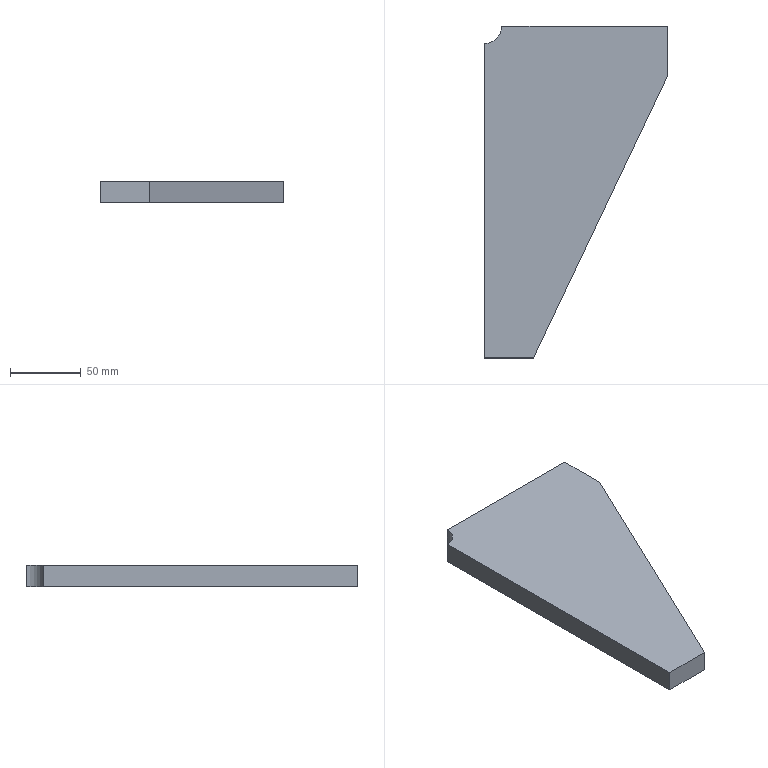Part | STEP file | Input 76 | 1 solid | 8 faces | box 130 x 235 x 15 mm | volume 313909 mm3 | plane 7 | cylinder 1 | commonest cylinder face diameters 25 x1
STEP:
#1=CARTESIAN_POINT('',(0.,0.,0.));
#2=DIRECTION('',(0.,0.,1.));
#3=DIRECTION('',(1.,0.,0.));
#4=AXIS2_PLACEMENT_3D('',#1,#2,#3);
#5=CARTESIAN_POINT('',(4022.,160.,7.5));
#6=VERTEX_POINT('',#5);
#7=CARTESIAN_POINT('',(4057.,160.,7.5));
#8=VERTEX_POINT('',#7);
#9=CARTESIAN_POINT('',(4057.,160.,7.5));
#10=DIRECTION('',(1.,0.,0.));
#11=VECTOR('',#10,1.);
#12=LINE('',#9,#11);
#13=CARTESIAN_POINT('',(4057.,160.,-7.5));
#14=DIRECTION('',(0.,-1.,0.));
#15=DIRECTION('',(1.,0.,0.));
#16=AXIS2_PLACEMENT_3D('',#13,#14,#15);
#17=PLANE('',#16);
#18=CARTESIAN_POINT('',(0.,15.));
#19=DIRECTION('',(1.,0.));
#20=VECTOR('',#19,1.);
#21=LINE('',#18,#20);
#22=(GEOMETRIC_REPRESENTATION_CONTEXT(2)PARAMETRIC_REPRESENTATION_CONTEXT()REPRESENTATION_CONTEXT('',''));
#23=DEFINITIONAL_REPRESENTATION('',(#21),#22);
#24=PCURVE('',#17,#23);
#25=CARTESIAN_POINT('',(4022.,395.,7.5));
#26=DIRECTION('',(0.,0.,1.));
#27=DIRECTION('',(1.,0.,0.));
#28=AXIS2_PLACEMENT_3D('',#25,#26,#27);
#29=PLANE('',#28);
#30=CARTESIAN_POINT('',(35.,-235.));
#31=DIRECTION('',(1.,0.));
#32=VECTOR('',#31,1.);
#33=LINE('',#30,#32);
#34=(GEOMETRIC_REPRESENTATION_CONTEXT(2)PARAMETRIC_REPRESENTATION_CONTEXT()REPRESENTATION_CONTEXT('',''));
#35=DEFINITIONAL_REPRESENTATION('',(#33),#34);
#36=PCURVE('',#29,#35);
#37=SURFACE_CURVE('',#12,(#24,#36),.PCURVE_S1.);
#38=EDGE_CURVE('',#6,#8,#37,.T.);
#39=ORIENTED_EDGE('',*,*,#38,.F.);
#40=CARTESIAN_POINT('',(4022.,160.,-7.5));
#41=VERTEX_POINT('',#40);
#42=CARTESIAN_POINT('',(4022.,160.,-7.5));
#43=DIRECTION('',(0.,0.,1.));
#44=VECTOR('',#43,1.);
#45=LINE('',#42,#44);
#46=CARTESIAN_POINT('',(-35.,0.));
#47=DIRECTION('',(0.,1.));
#48=VECTOR('',#47,1.);
#49=LINE('',#46,#48);
#50=(GEOMETRIC_REPRESENTATION_CONTEXT(2)PARAMETRIC_REPRESENTATION_CONTEXT()REPRESENTATION_CONTEXT('',''));
#51=DEFINITIONAL_REPRESENTATION('',(#49),#50);
#52=PCURVE('',#17,#51);
#53=CARTESIAN_POINT('',(4022.,160.,-7.5));
#54=DIRECTION('',(-1.,0.,0.));
#55=DIRECTION('',(0.,0.,1.));
#56=AXIS2_PLACEMENT_3D('',#53,#54,#55);
#57=PLANE('',#56);
#58=CARTESIAN_POINT('',(0.,0.));
#59=DIRECTION('',(1.,0.));
#60=VECTOR('',#59,1.);
#61=LINE('',#58,#60);
#62=(GEOMETRIC_REPRESENTATION_CONTEXT(2)PARAMETRIC_REPRESENTATION_CONTEXT()REPRESENTATION_CONTEXT('',''));
#63=DEFINITIONAL_REPRESENTATION('',(#61),#62);
#64=PCURVE('',#57,#63);
#65=SURFACE_CURVE('',#45,(#52,#64),.PCURVE_S1.);
#66=EDGE_CURVE('',#41,#6,#65,.T.);
#67=ORIENTED_EDGE('',*,*,#66,.F.);
#68=CARTESIAN_POINT('',(4057.,160.,-7.5));
#69=VERTEX_POINT('',#68);
#70=CARTESIAN_POINT('',(4057.,160.,-7.5));
#71=DIRECTION('',(1.,0.,0.));
#72=VECTOR('',#71,1.);
#73=LINE('',#70,#72);
#74=CARTESIAN_POINT('',(0.,0.));
#75=DIRECTION('',(1.,0.));
#76=VECTOR('',#75,1.);
#77=LINE('',#74,#76);
#78=(GEOMETRIC_REPRESENTATION_CONTEXT(2)PARAMETRIC_REPRESENTATION_CONTEXT()REPRESENTATION_CONTEXT('',''));
#79=DEFINITIONAL_REPRESENTATION('',(#77),#78);
#80=PCURVE('',#17,#79);
#81=CARTESIAN_POINT('',(4022.,395.,-7.5));
#82=DIRECTION('',(0.,0.,1.));
#83=DIRECTION('',(1.,0.,0.));
#84=AXIS2_PLACEMENT_3D('',#81,#82,#83);
#85=PLANE('',#84);
#86=CARTESIAN_POINT('',(35.,-235.));
#87=DIRECTION('',(1.,0.));
#88=VECTOR('',#87,1.);
#89=LINE('',#86,#88);
#90=(GEOMETRIC_REPRESENTATION_CONTEXT(2)PARAMETRIC_REPRESENTATION_CONTEXT()REPRESENTATION_CONTEXT('',''));
#91=DEFINITIONAL_REPRESENTATION('',(#89),#90);
#92=PCURVE('',#85,#91);
#93=SURFACE_CURVE('',#73,(#80,#92),.PCURVE_S1.);
#94=EDGE_CURVE('',#41,#69,#93,.T.);
#95=ORIENTED_EDGE('',*,*,#94,.T.);
#96=CARTESIAN_POINT('',(4057.,160.,-7.5));
#97=DIRECTION('',(0.,0.,1.));
#98=VECTOR('',#97,1.);
#99=LINE('',#96,#98);
#100=CARTESIAN_POINT('',(0.,0.));
#101=DIRECTION('',(0.,1.));
#102=VECTOR('',#101,1.);
#103=LINE('',#100,#102);
#104=(GEOMETRIC_REPRESENTATION_CONTEXT(2)PARAMETRIC_REPRESENTATION_CONTEXT()REPRESENTATION_CONTEXT('',''));
#105=DEFINITIONAL_REPRESENTATION('',(#103),#104);
#106=PCURVE('',#17,#105);
#107=CARTESIAN_POINT('',(4152.,360.,-7.5));
#108=DIRECTION('',(0.9033,-0.4291,0.));
#109=DIRECTION('',(0.4291,0.9033,0.));
#110=AXIS2_PLACEMENT_3D('',#107,#108,#109);
#111=PLANE('',#110);
#112=CARTESIAN_POINT('',(-221.416,0.));
#113=DIRECTION('',(0.,1.));
#114=VECTOR('',#113,1.);
#115=LINE('',#112,#114);
#116=(GEOMETRIC_REPRESENTATION_CONTEXT(2)PARAMETRIC_REPRESENTATION_CONTEXT()REPRESENTATION_CONTEXT('',''));
#117=DEFINITIONAL_REPRESENTATION('',(#115),#116);
#118=PCURVE('',#111,#117);
#119=SURFACE_CURVE('',#99,(#106,#118),.PCURVE_S1.);
#120=EDGE_CURVE('',#69,#8,#119,.T.);
#121=ORIENTED_EDGE('',*,*,#120,.T.);
#122=EDGE_LOOP('',(#39,#67,#95,#121));
#123=FACE_BOUND('',#122,.T.);
#124=ADVANCED_FACE('',(#123),#17,.T.);
#125=CARTESIAN_POINT('',(4022.,382.5,7.5));
#126=VERTEX_POINT('',#125);
#127=CARTESIAN_POINT('',(4022.,160.,7.5));
#128=DIRECTION('',(0.,-1.,0.));
#129=VECTOR('',#128,1.);
#130=LINE('',#127,#129);
#131=CARTESIAN_POINT('',(15.,0.));
#132=DIRECTION('',(0.,-1.));
#133=VECTOR('',#132,1.);
#134=LINE('',#131,#133);
#135=(GEOMETRIC_REPRESENTATION_CONTEXT(2)PARAMETRIC_REPRESENTATION_CONTEXT()REPRESENTATION_CONTEXT('',''));
#136=DEFINITIONAL_REPRESENTATION('',(#134),#135);
#137=PCURVE('',#57,#136);
#138=CARTESIAN_POINT('',(0.,-235.));
#139=DIRECTION('',(0.,-1.));
#140=VECTOR('',#139,1.);
#141=LINE('',#138,#140);
#142=(GEOMETRIC_REPRESENTATION_CONTEXT(2)PARAMETRIC_REPRESENTATION_CONTEXT()REPRESENTATION_CONTEXT('',''));
#143=DEFINITIONAL_REPRESENTATION('',(#141),#142);
#144=PCURVE('',#29,#143);
#145=SURFACE_CURVE('',#130,(#137,#144),.PCURVE_S1.);
#146=EDGE_CURVE('',#126,#6,#145,.T.);
#147=ORIENTED_EDGE('',*,*,#146,.F.);
#148=CARTESIAN_POINT('',(4022.,382.5,-7.5));
#149=VERTEX_POINT('',#148);
#150=CARTESIAN_POINT('',(4022.,382.5,-7.5));
#151=DIRECTION('',(0.,0.,1.));
#152=VECTOR('',#151,1.);
#153=LINE('',#150,#152);
#154=CARTESIAN_POINT('',(0.,222.5));
#155=DIRECTION('',(1.,0.));
#156=VECTOR('',#155,1.);
#157=LINE('',#154,#156);
#158=(GEOMETRIC_REPRESENTATION_CONTEXT(2)PARAMETRIC_REPRESENTATION_CONTEXT()REPRESENTATION_CONTEXT('',''));
#159=DEFINITIONAL_REPRESENTATION('',(#157),#158);
#160=PCURVE('',#57,#159);
#161=CARTESIAN_POINT('',(4022.,395.,-7.5));
#162=DIRECTION('',(0.,0.,1.));
#163=DIRECTION('',(1.,0.,0.));
#164=AXIS2_PLACEMENT_3D('',#161,#162,#163);
#165=CYLINDRICAL_SURFACE('',#164,12.5);
#166=CARTESIAN_POINT('',(4.712,0.));
#167=DIRECTION('',(0.,1.));
#168=VECTOR('',#167,1.);
#169=LINE('',#166,#168);
#170=(GEOMETRIC_REPRESENTATION_CONTEXT(2)PARAMETRIC_REPRESENTATION_CONTEXT()REPRESENTATION_CONTEXT('',''));
#171=DEFINITIONAL_REPRESENTATION('',(#169),#170);
#172=PCURVE('',#165,#171);
#173=SURFACE_CURVE('',#153,(#160,#172),.PCURVE_S1.);
#174=EDGE_CURVE('',#149,#126,#173,.T.);
#175=ORIENTED_EDGE('',*,*,#174,.F.);
#176=CARTESIAN_POINT('',(4022.,160.,-7.5));
#177=DIRECTION('',(0.,-1.,0.));
#178=VECTOR('',#177,1.);
#179=LINE('',#176,#178);
#180=CARTESIAN_POINT('',(0.,0.));
#181=DIRECTION('',(0.,-1.));
#182=VECTOR('',#181,1.);
#183=LINE('',#180,#182);
#184=(GEOMETRIC_REPRESENTATION_CONTEXT(2)PARAMETRIC_REPRESENTATION_CONTEXT()REPRESENTATION_CONTEXT('',''));
#185=DEFINITIONAL_REPRESENTATION('',(#183),#184);
#186=PCURVE('',#57,#185);
#187=CARTESIAN_POINT('',(0.,-235.));
#188=DIRECTION('',(0.,-1.));
#189=VECTOR('',#188,1.);
#190=LINE('',#187,#189);
#191=(GEOMETRIC_REPRESENTATION_CONTEXT(2)PARAMETRIC_REPRESENTATION_CONTEXT()REPRESENTATION_CONTEXT('',''));
#192=DEFINITIONAL_REPRESENTATION('',(#190),#191);
#193=PCURVE('',#85,#192);
#194=SURFACE_CURVE('',#179,(#186,#193),.PCURVE_S1.);
#195=EDGE_CURVE('',#149,#41,#194,.T.);
#196=ORIENTED_EDGE('',*,*,#195,.T.);
#197=ORIENTED_EDGE('',*,*,#66,.T.);
#198=EDGE_LOOP('',(#147,#175,#196,#197));
#199=FACE_BOUND('',#198,.T.);
#200=ADVANCED_FACE('',(#199),#57,.T.);
#201=ORIENTED_EDGE('',*,*,#174,.F.);
#202=CARTESIAN_POINT('',(4034.5,395.,-7.5));
#203=VERTEX_POINT('',#202);
#204=CARTESIAN_POINT('',(4022.,395.,-7.5));
#205=DIRECTION('',(0.,0.,-1.));
#206=DIRECTION('',(1.,0.,0.));
#207=AXIS2_PLACEMENT_3D('',#204,#205,#206);
#208=CIRCLE('',#207,12.5);
#209=CARTESIAN_POINT('',(6.283,0.));
#210=DIRECTION('',(-1.,0.));
#211=VECTOR('',#210,1.);
#212=LINE('',#209,#211);
#213=(GEOMETRIC_REPRESENTATION_CONTEXT(2)PARAMETRIC_REPRESENTATION_CONTEXT()REPRESENTATION_CONTEXT('',''));
#214=DEFINITIONAL_REPRESENTATION('',(#212),#213);
#215=PCURVE('',#165,#214);
#216=CARTESIAN_POINT('',(12.5,0.));
#217=CARTESIAN_POINT('',(12.5,-21.651));
#218=CARTESIAN_POINT('',(-6.25,-10.825));
#219=CARTESIAN_POINT('',(-25.,0.));
#220=CARTESIAN_POINT('',(-6.25,10.825));
#221=CARTESIAN_POINT('',(12.5,21.651));
#222=CARTESIAN_POINT('',(12.5,0.));
#223=(BOUNDED_CURVE()B_SPLINE_CURVE(2,(#216,#217,#218,#219,#220,#221,#222),.UNSPECIFIED.,.T.,.F.)B_SPLINE_CURVE_WITH_KNOTS((1,2,2,2,2,1),(-2.094,0.,2.094,4.189,6.283,8.378),.UNSPECIFIED.)CURVE()GEOMETRIC_REPRESENTATION_ITEM()RATIONAL_B_SPLINE_CURVE((1.,0.5,1.,0.5,1.,0.5,1.))REPRESENTATION_ITEM(''));
#224=(GEOMETRIC_REPRESENTATION_CONTEXT(2)PARAMETRIC_REPRESENTATION_CONTEXT()REPRESENTATION_CONTEXT('',''));
#225=DEFINITIONAL_REPRESENTATION('',(#223),#224);
#226=PCURVE('',#85,#225);
#227=SURFACE_CURVE('',#208,(#215,#226),.PCURVE_S1.);
#228=EDGE_CURVE('',#203,#149,#227,.T.);
#229=ORIENTED_EDGE('',*,*,#228,.F.);
#230=CARTESIAN_POINT('',(4034.5,395.,7.5));
#231=VERTEX_POINT('',#230);
#232=CARTESIAN_POINT('',(4034.5,395.,-7.5));
#233=DIRECTION('',(0.,0.,1.));
#234=VECTOR('',#233,1.);
#235=LINE('',#232,#234);
#236=CARTESIAN_POINT('',(6.283,0.));
#237=DIRECTION('',(0.,1.));
#238=VECTOR('',#237,1.);
#239=LINE('',#236,#238);
#240=(GEOMETRIC_REPRESENTATION_CONTEXT(2)PARAMETRIC_REPRESENTATION_CONTEXT()REPRESENTATION_CONTEXT('',''));
#241=DEFINITIONAL_REPRESENTATION('',(#239),#240);
#242=PCURVE('',#165,#241);
#243=CARTESIAN_POINT('',(4034.5,395.,-7.5));
#244=DIRECTION('',(0.,1.,0.));
#245=DIRECTION('',(0.,0.,1.));
#246=AXIS2_PLACEMENT_3D('',#243,#244,#245);
#247=PLANE('',#246);
#248=CARTESIAN_POINT('',(0.,0.));
#249=DIRECTION('',(1.,0.));
#250=VECTOR('',#249,1.);
#251=LINE('',#248,#250);
#252=(GEOMETRIC_REPRESENTATION_CONTEXT(2)PARAMETRIC_REPRESENTATION_CONTEXT()REPRESENTATION_CONTEXT('',''));
#253=DEFINITIONAL_REPRESENTATION('',(#251),#252);
#254=PCURVE('',#247,#253);
#255=SURFACE_CURVE('',#235,(#242,#254),.PCURVE_S1.);
#256=EDGE_CURVE('',#203,#231,#255,.T.);
#257=ORIENTED_EDGE('',*,*,#256,.T.);
#258=CARTESIAN_POINT('',(4022.,395.,7.5));
#259=DIRECTION('',(0.,0.,-1.));
#260=DIRECTION('',(1.,0.,0.));
#261=AXIS2_PLACEMENT_3D('',#258,#259,#260);
#262=CIRCLE('',#261,12.5);
#263=CARTESIAN_POINT('',(6.283,15.));
#264=DIRECTION('',(-1.,0.));
#265=VECTOR('',#264,1.);
#266=LINE('',#263,#265);
#267=(GEOMETRIC_REPRESENTATION_CONTEXT(2)PARAMETRIC_REPRESENTATION_CONTEXT()REPRESENTATION_CONTEXT('',''));
#268=DEFINITIONAL_REPRESENTATION('',(#266),#267);
#269=PCURVE('',#165,#268);
#270=CARTESIAN_POINT('',(12.5,0.));
#271=CARTESIAN_POINT('',(12.5,-21.651));
#272=CARTESIAN_POINT('',(-6.25,-10.825));
#273=CARTESIAN_POINT('',(-25.,0.));
#274=CARTESIAN_POINT('',(-6.25,10.825));
#275=CARTESIAN_POINT('',(12.5,21.651));
#276=CARTESIAN_POINT('',(12.5,0.));
#277=(BOUNDED_CURVE()B_SPLINE_CURVE(2,(#270,#271,#272,#273,#274,#275,#276),.UNSPECIFIED.,.T.,.F.)B_SPLINE_CURVE_WITH_KNOTS((1,2,2,2,2,1),(-2.094,0.,2.094,4.189,6.283,8.378),.UNSPECIFIED.)CURVE()GEOMETRIC_REPRESENTATION_ITEM()RATIONAL_B_SPLINE_CURVE((1.,0.5,1.,0.5,1.,0.5,1.))REPRESENTATION_ITEM(''));
#278=(GEOMETRIC_REPRESENTATION_CONTEXT(2)PARAMETRIC_REPRESENTATION_CONTEXT()REPRESENTATION_CONTEXT('',''));
#279=DEFINITIONAL_REPRESENTATION('',(#277),#278);
#280=PCURVE('',#29,#279);
#281=SURFACE_CURVE('',#262,(#269,#280),.PCURVE_S1.);
#282=EDGE_CURVE('',#231,#126,#281,.T.);
#283=ORIENTED_EDGE('',*,*,#282,.T.);
#284=EDGE_LOOP('',(#201,#229,#257,#283));
#285=FACE_BOUND('',#284,.F.);
#286=ADVANCED_FACE('',(#285),#165,.F.);
#287=CARTESIAN_POINT('',(4152.,395.,7.5));
#288=VERTEX_POINT('',#287);
#289=CARTESIAN_POINT('',(4034.5,395.,7.5));
#290=DIRECTION('',(-1.,0.,0.));
#291=VECTOR('',#290,1.);
#292=LINE('',#289,#291);
#293=CARTESIAN_POINT('',(15.,0.));
#294=DIRECTION('',(0.,-1.));
#295=VECTOR('',#294,1.);
#296=LINE('',#293,#295);
#297=(GEOMETRIC_REPRESENTATION_CONTEXT(2)PARAMETRIC_REPRESENTATION_CONTEXT()REPRESENTATION_CONTEXT('',''));
#298=DEFINITIONAL_REPRESENTATION('',(#296),#297);
#299=PCURVE('',#247,#298);
#300=CARTESIAN_POINT('',(12.5,0.));
#301=DIRECTION('',(-1.,0.));
#302=VECTOR('',#301,1.);
#303=LINE('',#300,#302);
#304=(GEOMETRIC_REPRESENTATION_CONTEXT(2)PARAMETRIC_REPRESENTATION_CONTEXT()REPRESENTATION_CONTEXT('',''));
#305=DEFINITIONAL_REPRESENTATION('',(#303),#304);
#306=PCURVE('',#29,#305);
#307=SURFACE_CURVE('',#292,(#299,#306),.PCURVE_S1.);
#308=EDGE_CURVE('',#288,#231,#307,.T.);
#309=ORIENTED_EDGE('',*,*,#308,.F.);
#310=CARTESIAN_POINT('',(4152.,395.,-7.5));
#311=VERTEX_POINT('',#310);
#312=CARTESIAN_POINT('',(4152.,395.,-7.5));
#313=DIRECTION('',(0.,0.,1.));
#314=VECTOR('',#313,1.);
#315=LINE('',#312,#314);
#316=CARTESIAN_POINT('',(0.,117.5));
#317=DIRECTION('',(1.,0.));
#318=VECTOR('',#317,1.);
#319=LINE('',#316,#318);
#320=(GEOMETRIC_REPRESENTATION_CONTEXT(2)PARAMETRIC_REPRESENTATION_CONTEXT()REPRESENTATION_CONTEXT('',''));
#321=DEFINITIONAL_REPRESENTATION('',(#319),#320);
#322=PCURVE('',#247,#321);
#323=CARTESIAN_POINT('',(4152.,395.,-7.5));
#324=DIRECTION('',(1.,0.,0.));
#325=DIRECTION('',(0.,1.,0.));
#326=AXIS2_PLACEMENT_3D('',#323,#324,#325);
#327=PLANE('',#326);
#328=CARTESIAN_POINT('',(0.,0.));
#329=DIRECTION('',(0.,1.));
#330=VECTOR('',#329,1.);
#331=LINE('',#328,#330);
#332=(GEOMETRIC_REPRESENTATION_CONTEXT(2)PARAMETRIC_REPRESENTATION_CONTEXT()REPRESENTATION_CONTEXT('',''));
#333=DEFINITIONAL_REPRESENTATION('',(#331),#332);
#334=PCURVE('',#327,#333);
#335=SURFACE_CURVE('',#315,(#322,#334),.PCURVE_S1.);
#336=EDGE_CURVE('',#311,#288,#335,.T.);
#337=ORIENTED_EDGE('',*,*,#336,.F.);
#338=CARTESIAN_POINT('',(4034.5,395.,-7.5));
#339=DIRECTION('',(-1.,0.,0.));
#340=VECTOR('',#339,1.);
#341=LINE('',#338,#340);
#342=CARTESIAN_POINT('',(0.,0.));
#343=DIRECTION('',(0.,-1.));
#344=VECTOR('',#343,1.);
#345=LINE('',#342,#344);
#346=(GEOMETRIC_REPRESENTATION_CONTEXT(2)PARAMETRIC_REPRESENTATION_CONTEXT()REPRESENTATION_CONTEXT('',''));
#347=DEFINITIONAL_REPRESENTATION('',(#345),#346);
#348=PCURVE('',#247,#347);
#349=CARTESIAN_POINT('',(12.5,0.));
#350=DIRECTION('',(-1.,0.));
#351=VECTOR('',#350,1.);
#352=LINE('',#349,#351);
#353=(GEOMETRIC_REPRESENTATION_CONTEXT(2)PARAMETRIC_REPRESENTATION_CONTEXT()REPRESENTATION_CONTEXT('',''));
#354=DEFINITIONAL_REPRESENTATION('',(#352),#353);
#355=PCURVE('',#85,#354);
#356=SURFACE_CURVE('',#341,(#348,#355),.PCURVE_S1.);
#357=EDGE_CURVE('',#311,#203,#356,.T.);
#358=ORIENTED_EDGE('',*,*,#357,.T.);
#359=ORIENTED_EDGE('',*,*,#256,.T.);
#360=EDGE_LOOP('',(#309,#337,#358,#359));
#361=FACE_BOUND('',#360,.T.);
#362=ADVANCED_FACE('',(#361),#247,.T.);
#363=CARTESIAN_POINT('',(4152.,360.,7.5));
#364=VERTEX_POINT('',#363);
#365=CARTESIAN_POINT('',(4152.,395.,7.5));
#366=DIRECTION('',(0.,1.,0.));
#367=VECTOR('',#366,1.);
#368=LINE('',#365,#367);
#369=CARTESIAN_POINT('',(0.,15.));
#370=DIRECTION('',(1.,0.));
#371=VECTOR('',#370,1.);
#372=LINE('',#369,#371);
#373=(GEOMETRIC_REPRESENTATION_CONTEXT(2)PARAMETRIC_REPRESENTATION_CONTEXT()REPRESENTATION_CONTEXT('',''));
#374=DEFINITIONAL_REPRESENTATION('',(#372),#373);
#375=PCURVE('',#327,#374);
#376=CARTESIAN_POINT('',(130.,0.));
#377=DIRECTION('',(0.,1.));
#378=VECTOR('',#377,1.);
#379=LINE('',#376,#378);
#380=(GEOMETRIC_REPRESENTATION_CONTEXT(2)PARAMETRIC_REPRESENTATION_CONTEXT()REPRESENTATION_CONTEXT('',''));
#381=DEFINITIONAL_REPRESENTATION('',(#379),#380);
#382=PCURVE('',#29,#381);
#383=SURFACE_CURVE('',#368,(#375,#382),.PCURVE_S1.);
#384=EDGE_CURVE('',#364,#288,#383,.T.);
#385=ORIENTED_EDGE('',*,*,#384,.F.);
#386=CARTESIAN_POINT('',(4152.,360.,-7.5));
#387=VERTEX_POINT('',#386);
#388=CARTESIAN_POINT('',(4152.,360.,-7.5));
#389=DIRECTION('',(0.,0.,1.));
#390=VECTOR('',#389,1.);
#391=LINE('',#388,#390);
#392=CARTESIAN_POINT('',(-35.,0.));
#393=DIRECTION('',(0.,1.));
#394=VECTOR('',#393,1.);
#395=LINE('',#392,#394);
#396=(GEOMETRIC_REPRESENTATION_CONTEXT(2)PARAMETRIC_REPRESENTATION_CONTEXT()REPRESENTATION_CONTEXT('',''));
#397=DEFINITIONAL_REPRESENTATION('',(#395),#396);
#398=PCURVE('',#327,#397);
#399=CARTESIAN_POINT('',(0.,0.));
#400=DIRECTION('',(0.,1.));
#401=VECTOR('',#400,1.);
#402=LINE('',#399,#401);
#403=(GEOMETRIC_REPRESENTATION_CONTEXT(2)PARAMETRIC_REPRESENTATION_CONTEXT()REPRESENTATION_CONTEXT('',''));
#404=DEFINITIONAL_REPRESENTATION('',(#402),#403);
#405=PCURVE('',#111,#404);
#406=SURFACE_CURVE('',#391,(#398,#405),.PCURVE_S1.);
#407=EDGE_CURVE('',#387,#364,#406,.T.);
#408=ORIENTED_EDGE('',*,*,#407,.F.);
#409=CARTESIAN_POINT('',(4152.,395.,-7.5));
#410=DIRECTION('',(0.,1.,0.));
#411=VECTOR('',#410,1.);
#412=LINE('',#409,#411);
#413=CARTESIAN_POINT('',(0.,0.));
#414=DIRECTION('',(1.,0.));
#415=VECTOR('',#414,1.);
#416=LINE('',#413,#415);
#417=(GEOMETRIC_REPRESENTATION_CONTEXT(2)PARAMETRIC_REPRESENTATION_CONTEXT()REPRESENTATION_CONTEXT('',''));
#418=DEFINITIONAL_REPRESENTATION('',(#416),#417);
#419=PCURVE('',#327,#418);
#420=CARTESIAN_POINT('',(130.,0.));
#421=DIRECTION('',(0.,1.));
#422=VECTOR('',#421,1.);
#423=LINE('',#420,#422);
#424=(GEOMETRIC_REPRESENTATION_CONTEXT(2)PARAMETRIC_REPRESENTATION_CONTEXT()REPRESENTATION_CONTEXT('',''));
#425=DEFINITIONAL_REPRESENTATION('',(#423),#424);
#426=PCURVE('',#85,#425);
#427=SURFACE_CURVE('',#412,(#419,#426),.PCURVE_S1.);
#428=EDGE_CURVE('',#387,#311,#427,.T.);
#429=ORIENTED_EDGE('',*,*,#428,.T.);
#430=ORIENTED_EDGE('',*,*,#336,.T.);
#431=EDGE_LOOP('',(#385,#408,#429,#430));
#432=FACE_BOUND('',#431,.T.);
#433=ADVANCED_FACE('',(#432),#327,.T.);
#434=CARTESIAN_POINT('',(4152.,360.,7.5));
#435=DIRECTION('',(0.4291,0.9033,0.));
#436=VECTOR('',#435,1.);
#437=LINE('',#434,#436);
#438=CARTESIAN_POINT('',(0.,15.));
#439=DIRECTION('',(1.,0.));
#440=VECTOR('',#439,1.);
#441=LINE('',#438,#440);
#442=(GEOMETRIC_REPRESENTATION_CONTEXT(2)PARAMETRIC_REPRESENTATION_CONTEXT()REPRESENTATION_CONTEXT('',''));
#443=DEFINITIONAL_REPRESENTATION('',(#441),#442);
#444=PCURVE('',#111,#443);
#445=CARTESIAN_POINT('',(130.,-35.));
#446=DIRECTION('',(0.4291,0.9033));
#447=VECTOR('',#446,1.);
#448=LINE('',#445,#447);
#449=(GEOMETRIC_REPRESENTATION_CONTEXT(2)PARAMETRIC_REPRESENTATION_CONTEXT()REPRESENTATION_CONTEXT('',''));
#450=DEFINITIONAL_REPRESENTATION('',(#448),#449);
#451=PCURVE('',#29,#450);
#452=SURFACE_CURVE('',#437,(#444,#451),.PCURVE_S1.);
#453=EDGE_CURVE('',#8,#364,#452,.T.);
#454=ORIENTED_EDGE('',*,*,#453,.F.);
#455=ORIENTED_EDGE('',*,*,#120,.F.);
#456=CARTESIAN_POINT('',(4152.,360.,-7.5));
#457=DIRECTION('',(0.4291,0.9033,0.));
#458=VECTOR('',#457,1.);
#459=LINE('',#456,#458);
#460=CARTESIAN_POINT('',(0.,0.));
#461=DIRECTION('',(1.,0.));
#462=VECTOR('',#461,1.);
#463=LINE('',#460,#462);
#464=(GEOMETRIC_REPRESENTATION_CONTEXT(2)PARAMETRIC_REPRESENTATION_CONTEXT()REPRESENTATION_CONTEXT('',''));
#465=DEFINITIONAL_REPRESENTATION('',(#463),#464);
#466=PCURVE('',#111,#465);
#467=CARTESIAN_POINT('',(130.,-35.));
#468=DIRECTION('',(0.4291,0.9033));
#469=VECTOR('',#468,1.);
#470=LINE('',#467,#469);
#471=(GEOMETRIC_REPRESENTATION_CONTEXT(2)PARAMETRIC_REPRESENTATION_CONTEXT()REPRESENTATION_CONTEXT('',''));
#472=DEFINITIONAL_REPRESENTATION('',(#470),#471);
#473=PCURVE('',#85,#472);
#474=SURFACE_CURVE('',#459,(#466,#473),.PCURVE_S1.);
#475=EDGE_CURVE('',#69,#387,#474,.T.);
#476=ORIENTED_EDGE('',*,*,#475,.T.);
#477=ORIENTED_EDGE('',*,*,#407,.T.);
#478=EDGE_LOOP('',(#454,#455,#476,#477));
#479=FACE_BOUND('',#478,.T.);
#480=ADVANCED_FACE('',(#479),#111,.T.);
#481=ORIENTED_EDGE('',*,*,#94,.F.);
#482=ORIENTED_EDGE('',*,*,#195,.F.);
#483=ORIENTED_EDGE('',*,*,#228,.F.);
#484=ORIENTED_EDGE('',*,*,#357,.F.);
#485=ORIENTED_EDGE('',*,*,#428,.F.);
#486=ORIENTED_EDGE('',*,*,#475,.F.);
#487=EDGE_LOOP('',(#481,#482,#483,#484,#485,#486));
#488=FACE_BOUND('',#487,.T.);
#489=ADVANCED_FACE('',(#488),#85,.F.);
#490=ORIENTED_EDGE('',*,*,#38,.T.);
#491=ORIENTED_EDGE('',*,*,#453,.T.);
#492=ORIENTED_EDGE('',*,*,#384,.T.);
#493=ORIENTED_EDGE('',*,*,#308,.T.);
#494=ORIENTED_EDGE('',*,*,#282,.T.);
#495=ORIENTED_EDGE('',*,*,#146,.T.);
#496=EDGE_LOOP('',(#490,#491,#492,#493,#494,#495));
#497=FACE_BOUND('',#496,.T.);
#498=ADVANCED_FACE('',(#497),#29,.T.);
#499=CLOSED_SHELL('',(#124,#200,#286,#362,#433,#480,#489,#498));
#500=MANIFOLD_SOLID_BREP('',#499);
#501=(LENGTH_UNIT()NAMED_UNIT(*)SI_UNIT(.MILLI.,.METRE.));
#502=UNCERTAINTY_MEASURE_WITH_UNIT(LENGTH_MEASURE(0.0000001),#501,'','');
#503=(NAMED_UNIT(*)PLANE_ANGLE_UNIT()SI_UNIT($,.RADIAN.));
#504=(NAMED_UNIT(*)SI_UNIT($,.STERADIAN.)SOLID_ANGLE_UNIT());
#505=(GEOMETRIC_REPRESENTATION_CONTEXT(3)GLOBAL_UNCERTAINTY_ASSIGNED_CONTEXT((#502))GLOBAL_UNIT_ASSIGNED_CONTEXT((#501,#503,#504))REPRESENTATION_CONTEXT('',''));
#506=ADVANCED_BREP_SHAPE_REPRESENTATION('',(#4,#500),#505);